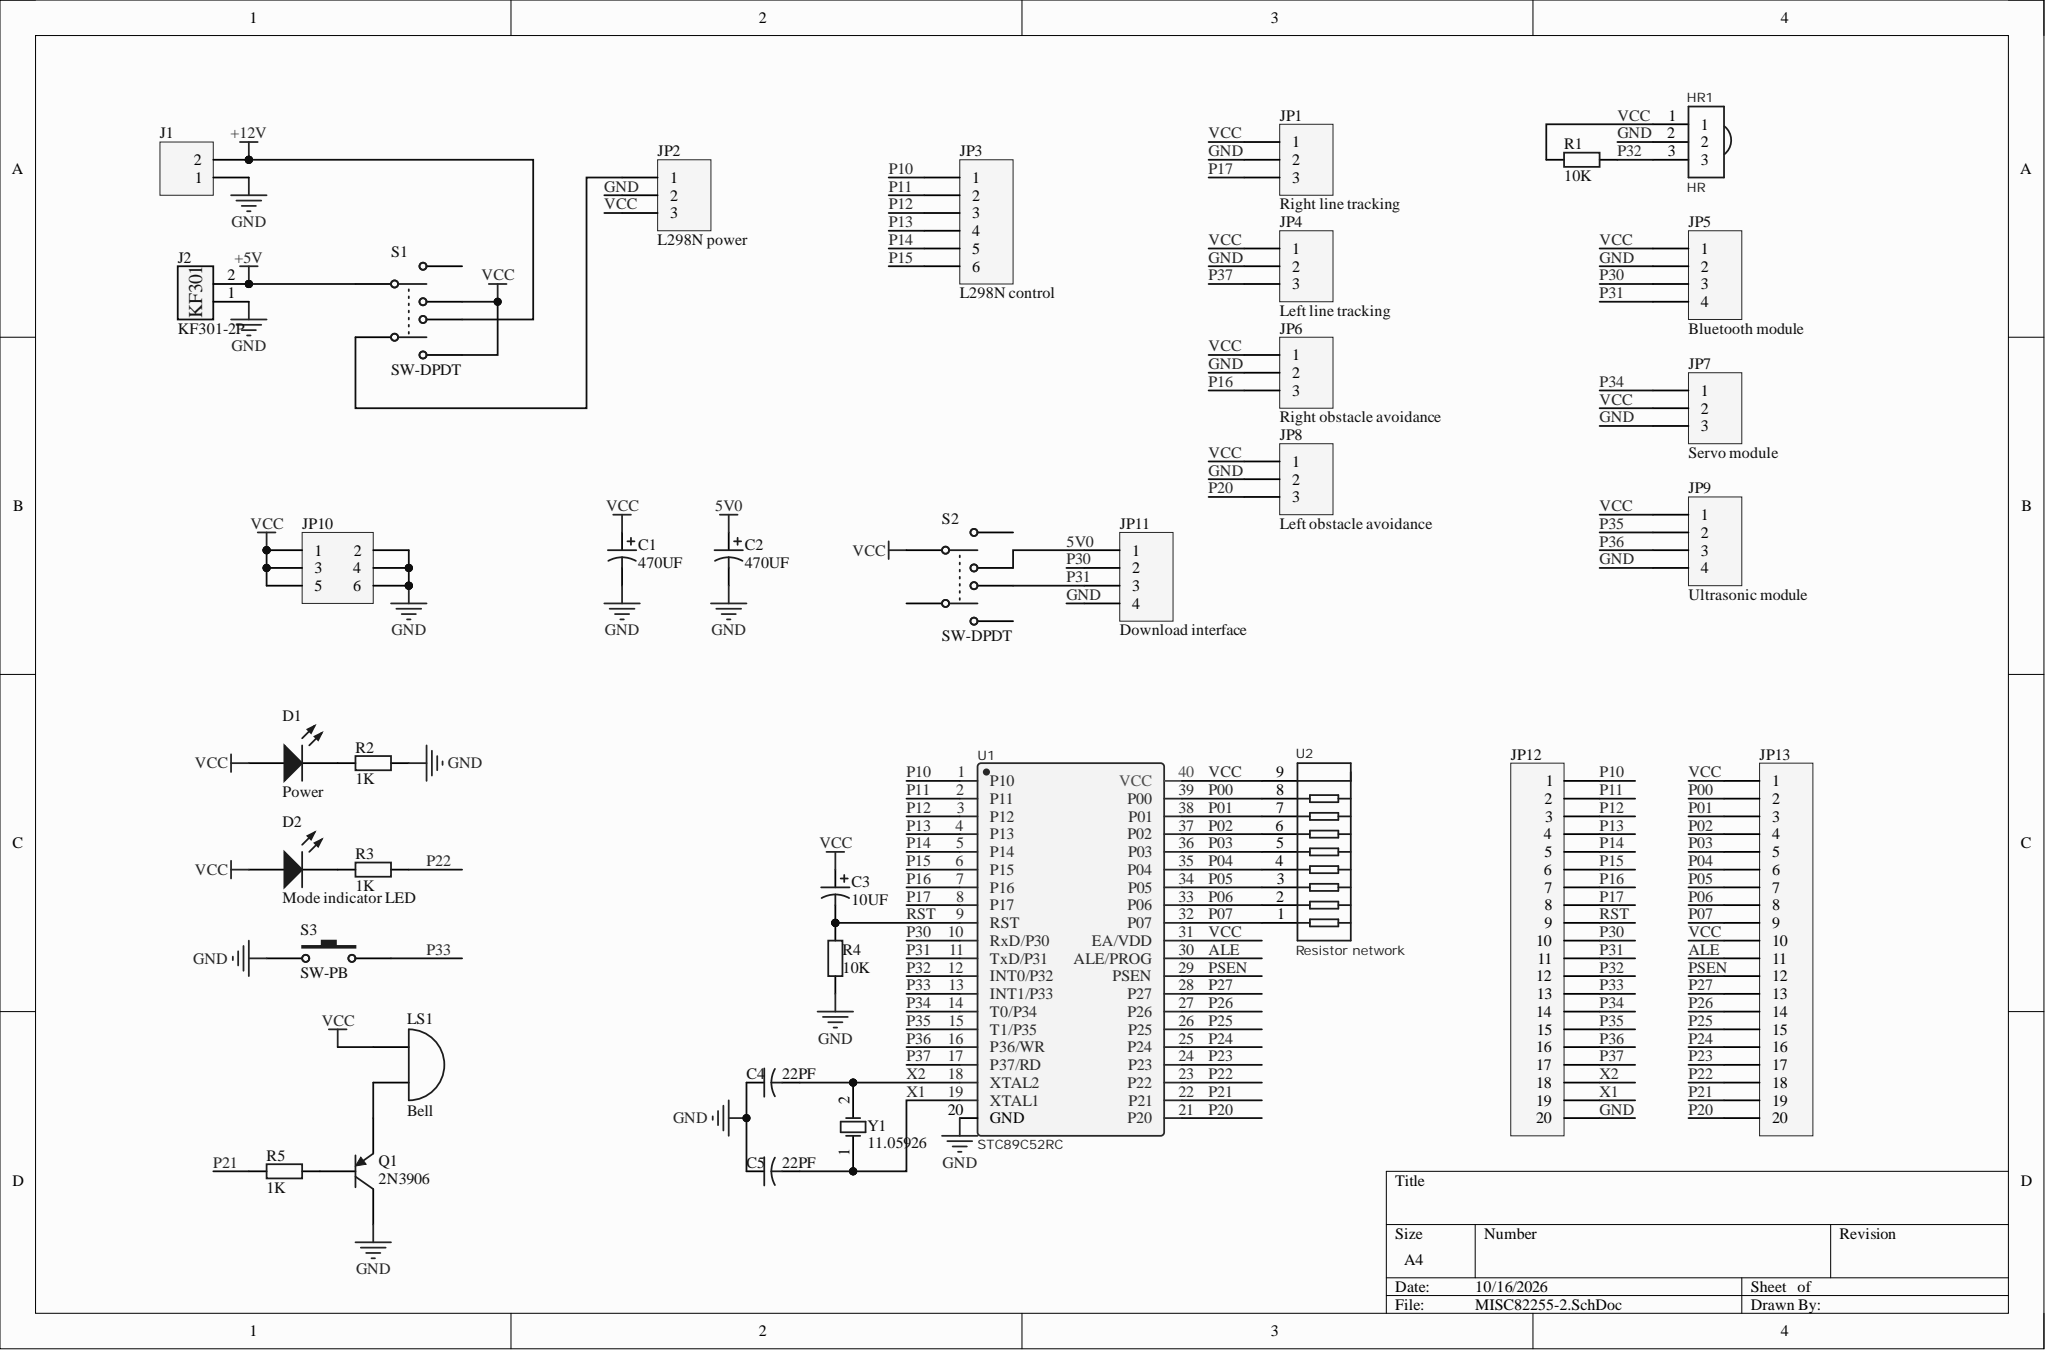Circuit board | Altium Designer | 36 parts | 47 nets
Bill of materials:
Comment,Description,Designator,Footprint,LibRef,Quantity
"470UF","Polarized Capacitor (Radial)","C1, C2","DR","Cap Pol1","2"
"10UF","Polarized Capacitor (Radial)","C3","DR","Cap Pol1","1"
"22PF","Capacitor","C4, C5","CAPR5-4X5","Cap2","2"
"Power","Typical RED GaAs LED","D1","LED-1","LED1","1"
"Mode indicator LED","Typical RED GaAs LED","D2","LED-1","LED1","1"
"HR","","HR1","SIP3","HR","1"
"Header 2","Header, 2-Pin","J1","HDR1X2","Header 2","1"
"KF301-2P","","J2","KF301-5.0-2P","KF301-2P","1"
"Right line tracking","Header, 3-Pin","JP1","HDR1X3","Header 3","1"
"L298N power","Header, 3-Pin","JP2","HDR1X3","Header 3","1"
"L298N control","Header, 6-Pin","JP3","HDR1X6","Header 6","1"
"Left line tracking","Header, 3-Pin","JP4","HDR1X3","Header 3","1"
"Bluetooth module","Header, 4-Pin","JP5","HDR1X4","Header 4","1"
"Right obstacle avoidance","Header, 3-Pin","JP6","HDR1X3","Header 3","1"
"Servo module","Header, 3-Pin","JP7","HDR1X3","Header 3","1"
"Left obstacle avoidance","Header, 3-Pin","JP8","HDR1X3","Header 3","1"
"Ultrasonic module","Header, 4-Pin","JP9","HDR1X4","Header 4","1"
"Header 3X2","Header, 3-Pin, Dual row","JP10","HDR2X3","Header 3X2","1"
"Download interface","Header, 4-Pin","JP11","HDR1X4","Header 4","1"
"Header 20","Header, 20-Pin","JP12, JP13","HDR1X20","Header 20","2"
"Bell","Electrical Bell","LS1","PIN2","Bell","1"
"2N3906","PNP General Purpose Amplifier","Q1","TO-92A","2N3906","1"
"10K","Resistor","R1, R4","AXIAL-0.4","Res2","2"
"1K","Resistor","R2, R3, R5","AXIAL-0.4","Res2","3"
"SW-DPDT","Double-Pole, Double-Throw Switch","S1, S2","DPDT-6","SW-DPDT","2"
"SW-PB","Switch","S3","SPST-2","SW-PB","1"
"STC89C52RC","","U1","STC89C52RC","STC89C52RC","1"
"Resistor network","","U2","paizu","排阻","1"
"11.059","Crystal Oscillator","Y1","R38","XTAL","1"
Netlist (Protel format):
[
C1
DR
470UF



]
[
C2
DR
470UF



]
[
C3
DR
10UF



]
[
C4
CAPR5-4X5
22PF



]
[
C5
CAPR5-4X5
22PF



]
[
D1
LED-1
Power



]
[
D2
LED-1
Mode indicator LED



]
[
HR1
SIP3
HR



]
[
J1
HDR1X2
Header 2



]
[
J2
KF301-5.0-2P
KF301-2P



]
[
JP1
HDR1X3
Right line tracking



]
[
JP2
HDR1X3
L298N power



]
[
JP3
HDR1X6
L298N control



]
[
JP4
HDR1X3
Left line tracking



]
[
JP5
HDR1X4
Bluetooth module



]
[
JP6
HDR1X3
Right obstacle avoidance



]
[
JP7
HDR1X3
Servo module



]
[
JP8
HDR1X3
Left obstacle avoidance



]
[
JP9
HDR1X4
Ultrasonic module



]
[
JP10
HDR2X3
Header 3X2



]
[
JP11
HDR1X4
Download interface



]
[
JP12
HDR1X20
Header 20



]
[
JP13
HDR1X20
Header 20



]
[
LS1
PIN2
Bell



]
[
Q1
TO-92A
2N3906



]
[
R1
AXIAL-0.4
10K



]
[
R2
AXIAL-0.4
1K



]
[
R3
AXIAL-0.4
1K



]
[
R4
AXIAL-0.4
10K



]
[
R5
AXIAL-0.4
1K



]
[
S1
DPDT-6
SW-DPDT



]
[
S2
DPDT-6
SW-DPDT



]
[
S3
SPST-2
SW-PB



]
[
U1
STC89C52RC
STC89C52RC



]
[
U2
paizu
Resistor network



]
[
Y1
R38
11.05926



]
(
X2
C4-2
JP12-18
U1-18
Y1-2
)
(
X1
C5-2
JP12-19
U1-19
Y1-1
)
(
VCC
C1-1
C3-1
D1-1
D2-1
HR1-1
JP1-1
JP2-3
JP4-1
JP5-1
JP6-1
JP7-2
JP8-1
JP9-1
JP10-1
JP10-3
JP10-5
JP13-1
JP13-10
LS1-1
R1-1
S1-3
S1-6
S2-1
U1-31
U1-40
U2-9
)
(
RST
C3-2
JP12-9
R4-2
U1-9
)
(
PSEN
JP13-12
U1-29
)
(
P37
JP4-3
JP12-17
U1-17
)
(
P36
JP9-3
JP12-16
U1-16
)
(
P35
JP9-2
JP12-15
U1-15
)
(
P34
JP7-1
JP12-14
U1-14
)
(
P33
JP12-13
S3-2
U1-13
)
(
P32
HR1-3
JP12-12
R1-2
U1-12
)
(
P31
JP5-4
JP11-3
JP12-11
S2-5
U1-11
)
(
P30
JP5-3
JP11-2
JP12-10
U1-10
)
(
P27
JP13-13
U1-28
)
(
P26
JP13-14
U1-27
)
(
P25
JP13-15
U1-26
)
(
P24
JP13-16
U1-25
)
(
P23
JP13-17
U1-24
)
(
P22
JP13-18
R3-2
U1-23
)
(
P21
JP13-19
R5-1
U1-22
)
(
P20
JP8-3
JP13-20
U1-21
)
(
P17
JP1-3
JP12-8
U1-8
)
(
P16
JP6-3
JP12-7
U1-7
)
(
P15
JP3-6
JP12-6
U1-6
)
(
P14
JP3-5
JP12-5
U1-5
)
(
P13
JP3-4
JP12-4
U1-4
)
(
P12
JP3-3
JP12-3
U1-3
)
(
P11
JP3-2
JP12-2
U1-2
)
(
P10
JP3-1
JP12-1
U1-1
)
(
P07
JP13-9
U1-32
U2-1
)
(
P06
JP13-8
U1-33
U2-2
)
(
P05
JP13-7
U1-34
U2-3
)
(
P04
JP13-6
U1-35
U2-4
)
(
P03
JP13-5
U1-36
U2-5
)
(
P02
JP13-4
U1-37
U2-6
)
(
P01
JP13-3
U1-38
U2-7
)
(
P00
JP13-2
U1-39
U2-8
)
(
NetQ1_2
Q1-2
R5-2
)
(
NetLS1_2
LS1-2
Q1-1
)
(
NetJP2_1
JP2-1
S1-4
)
(
NetD2_2
D2-2
R3-1
)
(
NetD1_2
D1-2
R2-1
)
(
GND
C1-2
C2-2
C4-1
C5-1
HR1-2
J1-1
J2-1
JP1-2
JP2-2
JP4-2
JP5-2
JP6-2
JP7-3
JP8-2
JP9-4
JP10-2
JP10-4
JP10-6
JP11-4
JP12-20
Q1-3
R2-2
R4-1
S3-1
U1-20
)
(
ALE
JP13-11
U1-30
)
(
+12V
J1-2
S1-5
)
(
+5V
J2-2
S1-1
)
(
5V0
C2-1
JP11-1
S2-3
)